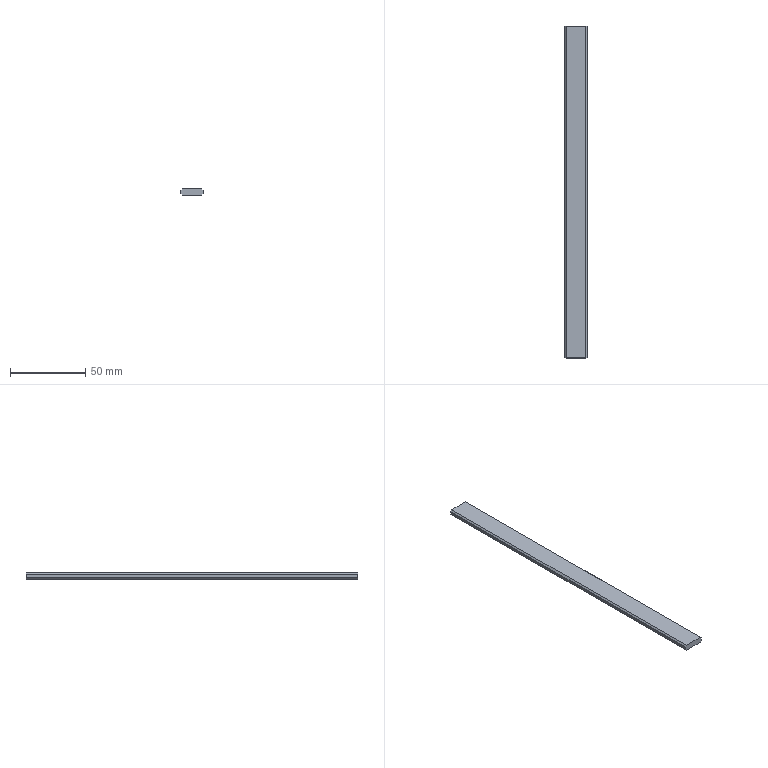Part | SolidWorks | features Chamfer 1, Extrusion 1 | 1 solid | 10 faces | box 15 x 220 x 4 mm | volume 12760 mm3 | plane 10
STEP:
#1=CARTESIAN_POINT('',(-7.5,110.,3.));
#2=VERTEX_POINT('',#1);
#3=CARTESIAN_POINT('',(-7.5,110.,1.));
#4=VERTEX_POINT('',#3);
#5=CARTESIAN_POINT('',(-7.5,110.,4.));
#6=DIRECTION('',(0.,0.,-1.));
#7=VECTOR('',#6,1000.);
#8=LINE('',#5,#7);
#9=EDGE_CURVE('',#2,#4,#8,.T.);
#10=ORIENTED_EDGE('',*,*,#9,.T.);
#11=CARTESIAN_POINT('',(-7.5,-110.,1.));
#12=VERTEX_POINT('',#11);
#13=CARTESIAN_POINT('',(-7.5,-110.,1.));
#14=DIRECTION('',(0.,-1.,0.));
#15=VECTOR('',#14,1000.);
#16=LINE('',#13,#15);
#17=EDGE_CURVE('',#4,#12,#16,.T.);
#18=ORIENTED_EDGE('',*,*,#17,.T.);
#19=CARTESIAN_POINT('',(-7.5,-110.,3.));
#20=VERTEX_POINT('',#19);
#21=CARTESIAN_POINT('',(-7.5,-110.,4.));
#22=DIRECTION('',(0.,0.,-1.));
#23=VECTOR('',#22,1000.);
#24=LINE('',#21,#23);
#25=EDGE_CURVE('',#20,#12,#24,.T.);
#26=ORIENTED_EDGE('',*,*,#25,.F.);
#27=CARTESIAN_POINT('',(-7.5,110.,3.));
#28=DIRECTION('',(0.,1.,0.));
#29=VECTOR('',#28,1000.);
#30=LINE('',#27,#29);
#31=EDGE_CURVE('',#20,#2,#30,.T.);
#32=ORIENTED_EDGE('',*,*,#31,.T.);
#33=EDGE_LOOP('',(#10,#18,#26,#32));
#34=FACE_OUTER_BOUND('',#33,.T.);
#35=CARTESIAN_POINT('',(-7.5,110.,4.));
#36=DIRECTION('',(1.,0.,0.));
#37=DIRECTION('',(0.,1.,0.));
#38=AXIS2_PLACEMENT_3D('',#35,#36,#37);
#39=PLANE('',#38);
#40=ADVANCED_FACE('',(#34),#39,.F.);
#41=ORIENTED_EDGE('',*,*,#25,.T.);
#42=CARTESIAN_POINT('',(-6.5,-110.,0.));
#43=VERTEX_POINT('',#42);
#44=CARTESIAN_POINT('',(-7.5,-110.,1.));
#45=DIRECTION('',(0.7071,0.,-0.7071));
#46=VECTOR('',#45,1000.);
#47=LINE('',#44,#46);
#48=EDGE_CURVE('',#12,#43,#47,.T.);
#49=ORIENTED_EDGE('',*,*,#48,.T.);
#50=CARTESIAN_POINT('',(6.5,-110.,0.));
#51=VERTEX_POINT('',#50);
#52=CARTESIAN_POINT('',(7.5,-110.,0.));
#53=DIRECTION('',(1.,0.,0.));
#54=VECTOR('',#53,1000.);
#55=LINE('',#52,#54);
#56=EDGE_CURVE('',#43,#51,#55,.T.);
#57=ORIENTED_EDGE('',*,*,#56,.T.);
#58=CARTESIAN_POINT('',(7.5,-110.,1.));
#59=VERTEX_POINT('',#58);
#60=CARTESIAN_POINT('',(7.5,-110.,1.));
#61=DIRECTION('',(0.7071,0.,0.7071));
#62=VECTOR('',#61,1000.);
#63=LINE('',#60,#62);
#64=EDGE_CURVE('',#51,#59,#63,.T.);
#65=ORIENTED_EDGE('',*,*,#64,.T.);
#66=CARTESIAN_POINT('',(7.5,-110.,3.));
#67=VERTEX_POINT('',#66);
#68=CARTESIAN_POINT('',(7.5,-110.,4.));
#69=DIRECTION('',(0.,0.,-1.));
#70=VECTOR('',#69,1000.);
#71=LINE('',#68,#70);
#72=EDGE_CURVE('',#67,#59,#71,.T.);
#73=ORIENTED_EDGE('',*,*,#72,.F.);
#74=CARTESIAN_POINT('',(6.5,-110.,4.));
#75=VERTEX_POINT('',#74);
#76=CARTESIAN_POINT('',(6.5,-110.,4.));
#77=DIRECTION('',(-0.7071,0.,0.7071));
#78=VECTOR('',#77,1000.);
#79=LINE('',#76,#78);
#80=EDGE_CURVE('',#67,#75,#79,.T.);
#81=ORIENTED_EDGE('',*,*,#80,.T.);
#82=CARTESIAN_POINT('',(-6.5,-110.,4.));
#83=VERTEX_POINT('',#82);
#84=CARTESIAN_POINT('',(7.5,-110.,4.));
#85=DIRECTION('',(1.,0.,0.));
#86=VECTOR('',#85,1000.);
#87=LINE('',#84,#86);
#88=EDGE_CURVE('',#83,#75,#87,.T.);
#89=ORIENTED_EDGE('',*,*,#88,.F.);
#90=CARTESIAN_POINT('',(-6.5,-110.,4.));
#91=DIRECTION('',(-0.7071,0.,-0.7071));
#92=VECTOR('',#91,1000.);
#93=LINE('',#90,#92);
#94=EDGE_CURVE('',#83,#20,#93,.T.);
#95=ORIENTED_EDGE('',*,*,#94,.T.);
#96=EDGE_LOOP('',(#41,#49,#57,#65,#73,#81,#89,#95));
#97=FACE_OUTER_BOUND('',#96,.T.);
#98=CARTESIAN_POINT('',(7.5,-110.,4.));
#99=DIRECTION('',(0.,1.,0.));
#100=DIRECTION('',(0.,0.,1.));
#101=AXIS2_PLACEMENT_3D('',#98,#99,#100);
#102=PLANE('',#101);
#103=ADVANCED_FACE('',(#97),#102,.F.);
#104=ORIENTED_EDGE('',*,*,#72,.T.);
#105=CARTESIAN_POINT('',(7.5,110.,1.));
#106=VERTEX_POINT('',#105);
#107=CARTESIAN_POINT('',(7.5,110.,1.));
#108=DIRECTION('',(0.,1.,0.));
#109=VECTOR('',#108,1000.);
#110=LINE('',#107,#109);
#111=EDGE_CURVE('',#59,#106,#110,.T.);
#112=ORIENTED_EDGE('',*,*,#111,.T.);
#113=CARTESIAN_POINT('',(7.5,110.,3.));
#114=VERTEX_POINT('',#113);
#115=CARTESIAN_POINT('',(7.5,110.,4.));
#116=DIRECTION('',(0.,0.,-1.));
#117=VECTOR('',#116,1000.);
#118=LINE('',#115,#117);
#119=EDGE_CURVE('',#114,#106,#118,.T.);
#120=ORIENTED_EDGE('',*,*,#119,.F.);
#121=CARTESIAN_POINT('',(7.5,110.,3.));
#122=DIRECTION('',(0.,-1.,0.));
#123=VECTOR('',#122,1000.);
#124=LINE('',#121,#123);
#125=EDGE_CURVE('',#114,#67,#124,.T.);
#126=ORIENTED_EDGE('',*,*,#125,.T.);
#127=EDGE_LOOP('',(#104,#112,#120,#126));
#128=FACE_OUTER_BOUND('',#127,.T.);
#129=CARTESIAN_POINT('',(7.5,110.,4.));
#130=DIRECTION('',(-1.,0.,0.));
#131=DIRECTION('',(0.,-1.,0.));
#132=AXIS2_PLACEMENT_3D('',#129,#130,#131);
#133=PLANE('',#132);
#134=ADVANCED_FACE('',(#128),#133,.F.);
#135=CARTESIAN_POINT('',(6.5,110.,0.));
#136=VERTEX_POINT('',#135);
#137=CARTESIAN_POINT('',(-6.5,110.,0.));
#138=VERTEX_POINT('',#137);
#139=CARTESIAN_POINT('',(7.5,110.,0.));
#140=DIRECTION('',(-1.,0.,0.));
#141=VECTOR('',#140,1000.);
#142=LINE('',#139,#141);
#143=EDGE_CURVE('',#136,#138,#142,.T.);
#144=ORIENTED_EDGE('',*,*,#143,.T.);
#145=CARTESIAN_POINT('',(-7.5,110.,1.));
#146=DIRECTION('',(-0.7071,0.,0.7071));
#147=VECTOR('',#146,1000.);
#148=LINE('',#145,#147);
#149=EDGE_CURVE('',#138,#4,#148,.T.);
#150=ORIENTED_EDGE('',*,*,#149,.T.);
#151=ORIENTED_EDGE('',*,*,#9,.F.);
#152=CARTESIAN_POINT('',(-6.5,110.,4.));
#153=VERTEX_POINT('',#152);
#154=CARTESIAN_POINT('',(-6.5,110.,4.));
#155=DIRECTION('',(0.7071,0.,0.7071));
#156=VECTOR('',#155,1000.);
#157=LINE('',#154,#156);
#158=EDGE_CURVE('',#2,#153,#157,.T.);
#159=ORIENTED_EDGE('',*,*,#158,.T.);
#160=CARTESIAN_POINT('',(6.5,110.,4.));
#161=VERTEX_POINT('',#160);
#162=CARTESIAN_POINT('',(7.5,110.,4.));
#163=DIRECTION('',(-1.,0.,0.));
#164=VECTOR('',#163,1000.);
#165=LINE('',#162,#164);
#166=EDGE_CURVE('',#161,#153,#165,.T.);
#167=ORIENTED_EDGE('',*,*,#166,.F.);
#168=CARTESIAN_POINT('',(6.5,110.,4.));
#169=DIRECTION('',(0.7071,0.,-0.7071));
#170=VECTOR('',#169,1000.);
#171=LINE('',#168,#170);
#172=EDGE_CURVE('',#161,#114,#171,.T.);
#173=ORIENTED_EDGE('',*,*,#172,.T.);
#174=ORIENTED_EDGE('',*,*,#119,.T.);
#175=CARTESIAN_POINT('',(7.5,110.,1.));
#176=DIRECTION('',(-0.7071,0.,-0.7071));
#177=VECTOR('',#176,1000.);
#178=LINE('',#175,#177);
#179=EDGE_CURVE('',#106,#136,#178,.T.);
#180=ORIENTED_EDGE('',*,*,#179,.T.);
#181=EDGE_LOOP('',(#144,#150,#151,#159,#167,#173,#174,#180));
#182=FACE_OUTER_BOUND('',#181,.T.);
#183=CARTESIAN_POINT('',(7.5,110.,4.));
#184=DIRECTION('',(0.,-1.,0.));
#185=DIRECTION('',(0.,0.,-1.));
#186=AXIS2_PLACEMENT_3D('',#183,#184,#185);
#187=PLANE('',#186);
#188=ADVANCED_FACE('',(#182),#187,.F.);
#189=ORIENTED_EDGE('',*,*,#166,.T.);
#190=CARTESIAN_POINT('',(-6.5,0.,4.));
#191=DIRECTION('',(0.,-1.,0.));
#192=VECTOR('',#191,1000.);
#193=LINE('',#190,#192);
#194=EDGE_CURVE('',#153,#83,#193,.T.);
#195=ORIENTED_EDGE('',*,*,#194,.T.);
#196=ORIENTED_EDGE('',*,*,#88,.T.);
#197=CARTESIAN_POINT('',(6.5,0.,4.));
#198=DIRECTION('',(0.,1.,0.));
#199=VECTOR('',#198,1000.);
#200=LINE('',#197,#199);
#201=EDGE_CURVE('',#75,#161,#200,.T.);
#202=ORIENTED_EDGE('',*,*,#201,.T.);
#203=EDGE_LOOP('',(#189,#195,#196,#202));
#204=FACE_OUTER_BOUND('',#203,.T.);
#205=CARTESIAN_POINT('',(0.,0.,4.));
#206=DIRECTION('',(0.,0.,-1.));
#207=DIRECTION('',(-1.,0.,0.));
#208=AXIS2_PLACEMENT_3D('',#205,#206,#207);
#209=PLANE('',#208);
#210=ADVANCED_FACE('',(#204),#209,.F.);
#211=ORIENTED_EDGE('',*,*,#56,.F.);
#212=CARTESIAN_POINT('',(-6.5,110.,0.));
#213=DIRECTION('',(0.,1.,0.));
#214=VECTOR('',#213,1000.);
#215=LINE('',#212,#214);
#216=EDGE_CURVE('',#43,#138,#215,.T.);
#217=ORIENTED_EDGE('',*,*,#216,.T.);
#218=ORIENTED_EDGE('',*,*,#143,.F.);
#219=CARTESIAN_POINT('',(6.5,-110.,0.));
#220=DIRECTION('',(0.,-1.,0.));
#221=VECTOR('',#220,1000.);
#222=LINE('',#219,#221);
#223=EDGE_CURVE('',#136,#51,#222,.T.);
#224=ORIENTED_EDGE('',*,*,#223,.T.);
#225=EDGE_LOOP('',(#211,#217,#218,#224));
#226=FACE_OUTER_BOUND('',#225,.T.);
#227=CARTESIAN_POINT('',(0.,0.,0.));
#228=DIRECTION('',(0.,0.,-1.));
#229=DIRECTION('',(-1.,0.,0.));
#230=AXIS2_PLACEMENT_3D('',#227,#228,#229);
#231=PLANE('',#230);
#232=ADVANCED_FACE('',(#226),#231,.T.);
#233=ORIENTED_EDGE('',*,*,#149,.F.);
#234=ORIENTED_EDGE('',*,*,#216,.F.);
#235=ORIENTED_EDGE('',*,*,#48,.F.);
#236=ORIENTED_EDGE('',*,*,#17,.F.);
#237=EDGE_LOOP('',(#233,#234,#235,#236));
#238=FACE_OUTER_BOUND('',#237,.T.);
#239=CARTESIAN_POINT('',(-7.5,110.,1.));
#240=DIRECTION('',(-0.7071,0.,-0.7071));
#241=DIRECTION('',(0.,1.,0.));
#242=AXIS2_PLACEMENT_3D('',#239,#240,#241);
#243=PLANE('',#242);
#244=ADVANCED_FACE('',(#238),#243,.T.);
#245=ORIENTED_EDGE('',*,*,#64,.F.);
#246=ORIENTED_EDGE('',*,*,#223,.F.);
#247=ORIENTED_EDGE('',*,*,#179,.F.);
#248=ORIENTED_EDGE('',*,*,#111,.F.);
#249=EDGE_LOOP('',(#245,#246,#247,#248));
#250=FACE_OUTER_BOUND('',#249,.T.);
#251=CARTESIAN_POINT('',(7.5,110.,1.));
#252=DIRECTION('',(0.7071,0.,-0.7071));
#253=DIRECTION('',(0.,-1.,0.));
#254=AXIS2_PLACEMENT_3D('',#251,#252,#253);
#255=PLANE('',#254);
#256=ADVANCED_FACE('',(#250),#255,.T.);
#257=ORIENTED_EDGE('',*,*,#158,.F.);
#258=ORIENTED_EDGE('',*,*,#31,.F.);
#259=ORIENTED_EDGE('',*,*,#94,.F.);
#260=ORIENTED_EDGE('',*,*,#194,.F.);
#261=EDGE_LOOP('',(#257,#258,#259,#260));
#262=FACE_OUTER_BOUND('',#261,.T.);
#263=CARTESIAN_POINT('',(-6.5,0.,4.));
#264=DIRECTION('',(0.7071,0.,-0.7071));
#265=DIRECTION('',(0.,-1.,0.));
#266=AXIS2_PLACEMENT_3D('',#263,#264,#265);
#267=PLANE('',#266);
#268=ADVANCED_FACE('',(#262),#267,.F.);
#269=ORIENTED_EDGE('',*,*,#80,.F.);
#270=ORIENTED_EDGE('',*,*,#125,.F.);
#271=ORIENTED_EDGE('',*,*,#172,.F.);
#272=ORIENTED_EDGE('',*,*,#201,.F.);
#273=EDGE_LOOP('',(#269,#270,#271,#272));
#274=FACE_OUTER_BOUND('',#273,.T.);
#275=CARTESIAN_POINT('',(6.5,0.,4.));
#276=DIRECTION('',(-0.7071,0.,-0.7071));
#277=DIRECTION('',(0.,1.,0.));
#278=AXIS2_PLACEMENT_3D('',#275,#276,#277);
#279=PLANE('',#278);
#280=ADVANCED_FACE('',(#274),#279,.F.);
#281=CLOSED_SHELL('',(#40,#103,#134,#188,#210,#232,#244,#256,#268,#280));
#282=MANIFOLD_SOLID_BREP('',#281);
#283=CARTESIAN_POINT('',(0.,0.,0.));
#284=DIRECTION('',(0.,0.,1.));
#285=DIRECTION('',(1.,0.,0.));
#286=AXIS2_PLACEMENT_3D('',#283,#284,#285);
#287=(LENGTH_UNIT()NAMED_UNIT(*)SI_UNIT(.MILLI.,.METRE.));
#288=UNCERTAINTY_MEASURE_WITH_UNIT(LENGTH_MEASURE(0.00001),#287,'','');
#289=(NAMED_UNIT(*)PLANE_ANGLE_UNIT()SI_UNIT($,.RADIAN.));
#290=(NAMED_UNIT(*)SI_UNIT($,.STERADIAN.)SOLID_ANGLE_UNIT());
#291=(GEOMETRIC_REPRESENTATION_CONTEXT(3)GLOBAL_UNCERTAINTY_ASSIGNED_CONTEXT((#288))GLOBAL_UNIT_ASSIGNED_CONTEXT((#287,#289,#290))REPRESENTATION_CONTEXT('',''));
#292=ADVANCED_BREP_SHAPE_REPRESENTATION('',(#282,#286),#291);